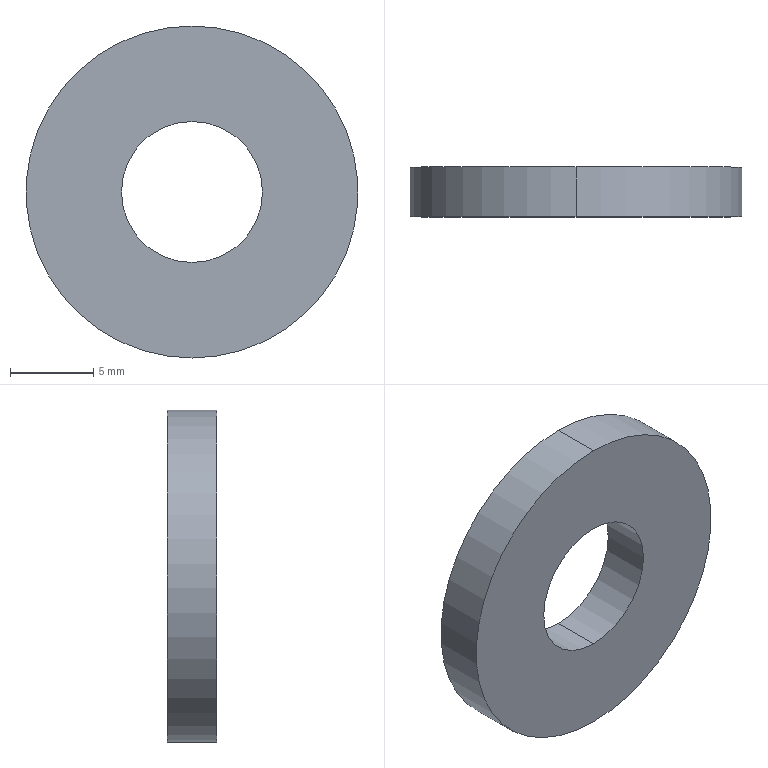Part | SolidWorks | features Extrusion 1 | 1 solid | 6 faces | box 20 x 3 x 20 mm | volume 772.243 mm3 | cylinder 4 | plane 2 | commonest cylinder face diameters 8.5 x2 20 x2
STEP:
#1=CARTESIAN_POINT('',(0.,3.,-4.25));
#2=VERTEX_POINT('',#1);
#3=CARTESIAN_POINT('',(0.,3.,4.25));
#4=VERTEX_POINT('',#3);
#5=CARTESIAN_POINT('',(0.,3.,0.));
#6=DIRECTION('',(0.,1.,0.));
#7=DIRECTION('',(0.,0.,1.));
#8=AXIS2_PLACEMENT_3D('',#5,#6,#7);
#9=CIRCLE('',#8,4.25);
#10=EDGE_CURVE('',#2,#4,#9,.T.);
#11=ORIENTED_EDGE('',*,*,#10,.T.);
#12=CARTESIAN_POINT('',(0.,0.,4.25));
#13=VERTEX_POINT('',#12);
#14=CARTESIAN_POINT('',(0.,3.,4.25));
#15=DIRECTION('',(0.,-1.,0.));
#16=VECTOR('',#15,1000.);
#17=LINE('',#14,#16);
#18=EDGE_CURVE('',#4,#13,#17,.T.);
#19=ORIENTED_EDGE('',*,*,#18,.T.);
#20=CARTESIAN_POINT('',(0.,0.,-4.25));
#21=VERTEX_POINT('',#20);
#22=CARTESIAN_POINT('',(0.,0.,0.));
#23=DIRECTION('',(0.,1.,0.));
#24=DIRECTION('',(0.,0.,1.));
#25=AXIS2_PLACEMENT_3D('',#22,#23,#24);
#26=CIRCLE('',#25,4.25);
#27=EDGE_CURVE('',#21,#13,#26,.T.);
#28=ORIENTED_EDGE('',*,*,#27,.F.);
#29=CARTESIAN_POINT('',(0.,3.,-4.25));
#30=DIRECTION('',(0.,-1.,0.));
#31=VECTOR('',#30,1000.);
#32=LINE('',#29,#31);
#33=EDGE_CURVE('',#2,#21,#32,.T.);
#34=ORIENTED_EDGE('',*,*,#33,.F.);
#35=EDGE_LOOP('',(#11,#19,#28,#34));
#36=FACE_OUTER_BOUND('',#35,.T.);
#37=CARTESIAN_POINT('',(0.,3.,0.));
#38=DIRECTION('',(0.,-1.,0.));
#39=DIRECTION('',(0.,0.,-1.));
#40=AXIS2_PLACEMENT_3D('',#37,#38,#39);
#41=CYLINDRICAL_SURFACE('',#40,4.25);
#42=ADVANCED_FACE('',(#36),#41,.F.);
#43=CARTESIAN_POINT('',(0.,3.,10.));
#44=VERTEX_POINT('',#43);
#45=CARTESIAN_POINT('',(0.,3.,-10.));
#46=VERTEX_POINT('',#45);
#47=CARTESIAN_POINT('',(0.,3.,0.));
#48=DIRECTION('',(0.,1.,0.));
#49=DIRECTION('',(0.,0.,1.));
#50=AXIS2_PLACEMENT_3D('',#47,#48,#49);
#51=CIRCLE('',#50,10.);
#52=EDGE_CURVE('',#44,#46,#51,.T.);
#53=ORIENTED_EDGE('',*,*,#52,.F.);
#54=CARTESIAN_POINT('',(0.,0.,10.));
#55=VERTEX_POINT('',#54);
#56=CARTESIAN_POINT('',(0.,3.,10.));
#57=DIRECTION('',(0.,-1.,0.));
#58=VECTOR('',#57,1000.);
#59=LINE('',#56,#58);
#60=EDGE_CURVE('',#44,#55,#59,.T.);
#61=ORIENTED_EDGE('',*,*,#60,.T.);
#62=CARTESIAN_POINT('',(0.,0.,-10.));
#63=VERTEX_POINT('',#62);
#64=CARTESIAN_POINT('',(0.,0.,0.));
#65=DIRECTION('',(0.,1.,0.));
#66=DIRECTION('',(0.,0.,1.));
#67=AXIS2_PLACEMENT_3D('',#64,#65,#66);
#68=CIRCLE('',#67,10.);
#69=EDGE_CURVE('',#55,#63,#68,.T.);
#70=ORIENTED_EDGE('',*,*,#69,.T.);
#71=CARTESIAN_POINT('',(0.,3.,-10.));
#72=DIRECTION('',(0.,-1.,0.));
#73=VECTOR('',#72,1000.);
#74=LINE('',#71,#73);
#75=EDGE_CURVE('',#46,#63,#74,.T.);
#76=ORIENTED_EDGE('',*,*,#75,.F.);
#77=EDGE_LOOP('',(#53,#61,#70,#76));
#78=FACE_OUTER_BOUND('',#77,.T.);
#79=CARTESIAN_POINT('',(0.,3.,0.));
#80=DIRECTION('',(0.,-1.,0.));
#81=DIRECTION('',(0.,0.,-1.));
#82=AXIS2_PLACEMENT_3D('',#79,#80,#81);
#83=CYLINDRICAL_SURFACE('',#82,10.);
#84=ADVANCED_FACE('',(#78),#83,.T.);
#85=CARTESIAN_POINT('',(0.,3.,0.));
#86=DIRECTION('',(0.,1.,0.));
#87=DIRECTION('',(0.,0.,1.));
#88=AXIS2_PLACEMENT_3D('',#85,#86,#87);
#89=CIRCLE('',#88,10.);
#90=EDGE_CURVE('',#46,#44,#89,.T.);
#91=ORIENTED_EDGE('',*,*,#90,.T.);
#92=ORIENTED_EDGE('',*,*,#52,.T.);
#93=EDGE_LOOP('',(#91,#92));
#94=FACE_OUTER_BOUND('',#93,.T.);
#95=ORIENTED_EDGE('',*,*,#10,.F.);
#96=CARTESIAN_POINT('',(0.,3.,0.));
#97=DIRECTION('',(0.,1.,0.));
#98=DIRECTION('',(0.,0.,1.));
#99=AXIS2_PLACEMENT_3D('',#96,#97,#98);
#100=CIRCLE('',#99,4.25);
#101=EDGE_CURVE('',#4,#2,#100,.T.);
#102=ORIENTED_EDGE('',*,*,#101,.F.);
#103=EDGE_LOOP('',(#95,#102));
#104=FACE_BOUND('',#103,.T.);
#105=CARTESIAN_POINT('',(0.,3.,0.));
#106=DIRECTION('',(0.,1.,0.));
#107=DIRECTION('',(0.,0.,1.));
#108=AXIS2_PLACEMENT_3D('',#105,#106,#107);
#109=PLANE('',#108);
#110=ADVANCED_FACE('',(#94,#104),#109,.T.);
#111=CARTESIAN_POINT('',(0.,0.,0.));
#112=DIRECTION('',(0.,1.,0.));
#113=DIRECTION('',(0.,0.,1.));
#114=AXIS2_PLACEMENT_3D('',#111,#112,#113);
#115=CIRCLE('',#114,10.);
#116=EDGE_CURVE('',#63,#55,#115,.T.);
#117=ORIENTED_EDGE('',*,*,#116,.F.);
#118=ORIENTED_EDGE('',*,*,#69,.F.);
#119=EDGE_LOOP('',(#117,#118));
#120=FACE_OUTER_BOUND('',#119,.T.);
#121=ORIENTED_EDGE('',*,*,#27,.T.);
#122=CARTESIAN_POINT('',(0.,0.,0.));
#123=DIRECTION('',(0.,1.,0.));
#124=DIRECTION('',(0.,0.,1.));
#125=AXIS2_PLACEMENT_3D('',#122,#123,#124);
#126=CIRCLE('',#125,4.25);
#127=EDGE_CURVE('',#13,#21,#126,.T.);
#128=ORIENTED_EDGE('',*,*,#127,.T.);
#129=EDGE_LOOP('',(#121,#128));
#130=FACE_BOUND('',#129,.T.);
#131=CARTESIAN_POINT('',(0.,0.,0.));
#132=DIRECTION('',(0.,1.,0.));
#133=DIRECTION('',(0.,0.,1.));
#134=AXIS2_PLACEMENT_3D('',#131,#132,#133);
#135=PLANE('',#134);
#136=ADVANCED_FACE('',(#120,#130),#135,.F.);
#137=ORIENTED_EDGE('',*,*,#60,.F.);
#138=ORIENTED_EDGE('',*,*,#90,.F.);
#139=ORIENTED_EDGE('',*,*,#75,.T.);
#140=ORIENTED_EDGE('',*,*,#116,.T.);
#141=EDGE_LOOP('',(#137,#138,#139,#140));
#142=FACE_OUTER_BOUND('',#141,.T.);
#143=CARTESIAN_POINT('',(0.,3.,0.));
#144=DIRECTION('',(0.,-1.,0.));
#145=DIRECTION('',(0.,0.,-1.));
#146=AXIS2_PLACEMENT_3D('',#143,#144,#145);
#147=CYLINDRICAL_SURFACE('',#146,10.);
#148=ADVANCED_FACE('',(#142),#147,.T.);
#149=ORIENTED_EDGE('',*,*,#18,.F.);
#150=ORIENTED_EDGE('',*,*,#101,.T.);
#151=ORIENTED_EDGE('',*,*,#33,.T.);
#152=ORIENTED_EDGE('',*,*,#127,.F.);
#153=EDGE_LOOP('',(#149,#150,#151,#152));
#154=FACE_OUTER_BOUND('',#153,.T.);
#155=CARTESIAN_POINT('',(0.,3.,0.));
#156=DIRECTION('',(0.,-1.,0.));
#157=DIRECTION('',(0.,0.,-1.));
#158=AXIS2_PLACEMENT_3D('',#155,#156,#157);
#159=CYLINDRICAL_SURFACE('',#158,4.25);
#160=ADVANCED_FACE('',(#154),#159,.F.);
#161=CLOSED_SHELL('',(#42,#84,#110,#136,#148,#160));
#162=MANIFOLD_SOLID_BREP('',#161);
#163=CARTESIAN_POINT('',(0.,0.,0.));
#164=DIRECTION('',(0.,0.,1.));
#165=DIRECTION('',(1.,0.,0.));
#166=AXIS2_PLACEMENT_3D('',#163,#164,#165);
#167=(LENGTH_UNIT()NAMED_UNIT(*)SI_UNIT(.MILLI.,.METRE.));
#168=UNCERTAINTY_MEASURE_WITH_UNIT(LENGTH_MEASURE(0.00001),#167,'','');
#169=(NAMED_UNIT(*)PLANE_ANGLE_UNIT()SI_UNIT($,.RADIAN.));
#170=(NAMED_UNIT(*)SI_UNIT($,.STERADIAN.)SOLID_ANGLE_UNIT());
#171=(GEOMETRIC_REPRESENTATION_CONTEXT(3)GLOBAL_UNCERTAINTY_ASSIGNED_CONTEXT((#168))GLOBAL_UNIT_ASSIGNED_CONTEXT((#167,#169,#170))REPRESENTATION_CONTEXT('',''));
#172=ADVANCED_BREP_SHAPE_REPRESENTATION('',(#162,#166),#171);